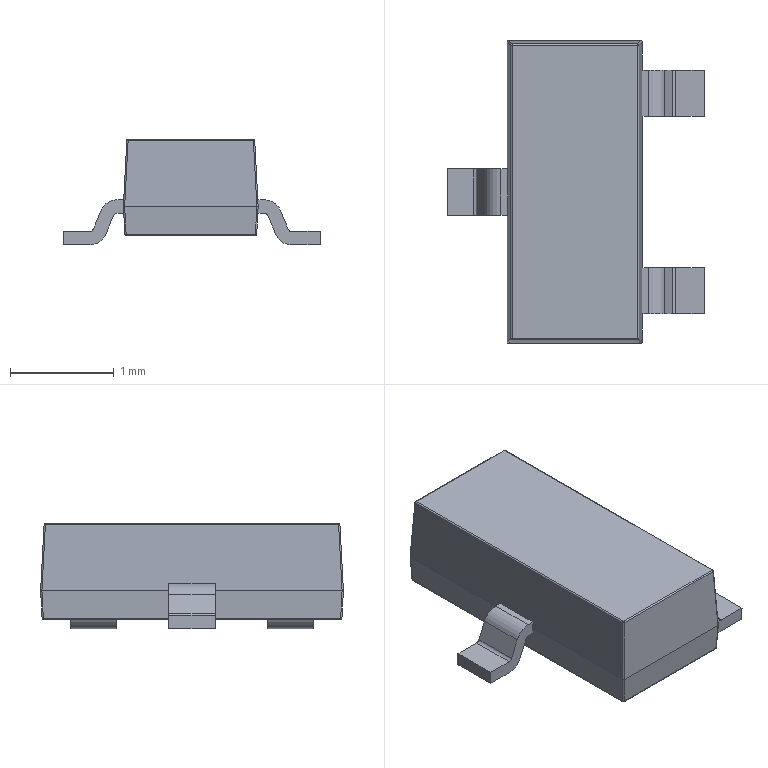Part | STEP file | RJ-USIO-V1_2-220411_45 | 1 solid | 73 faces | box 2.476 x 2.92 x 1.02 mm | volume 3.553 mm3 | plane 37 | cylinder 28 | sphere 8 | commonest cylinder face diameters 0.025 x16 0.07 x6 0.33 x6